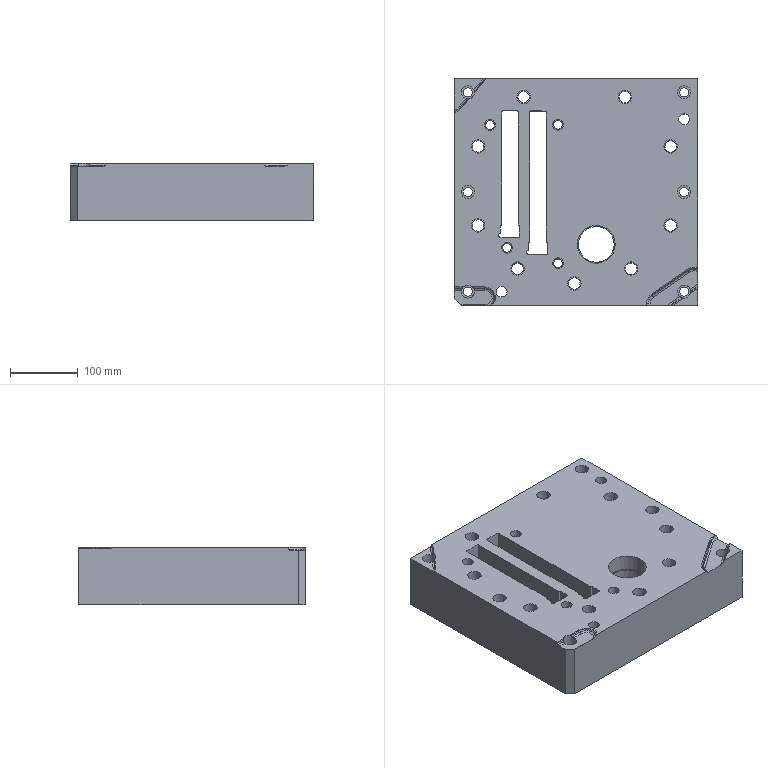Part | NX | features solid 2 | 1 solid | 115 faces | box 360.002 x 335.002 x 85 mm | volume 8720079 mm3 | cylinder 57 | plane 40 | spline 14 | cone 4 | commonest cylinder face diameters 17 x9 20 x9 6.2 x8 3.2 x7 13.5 x6 16 x6